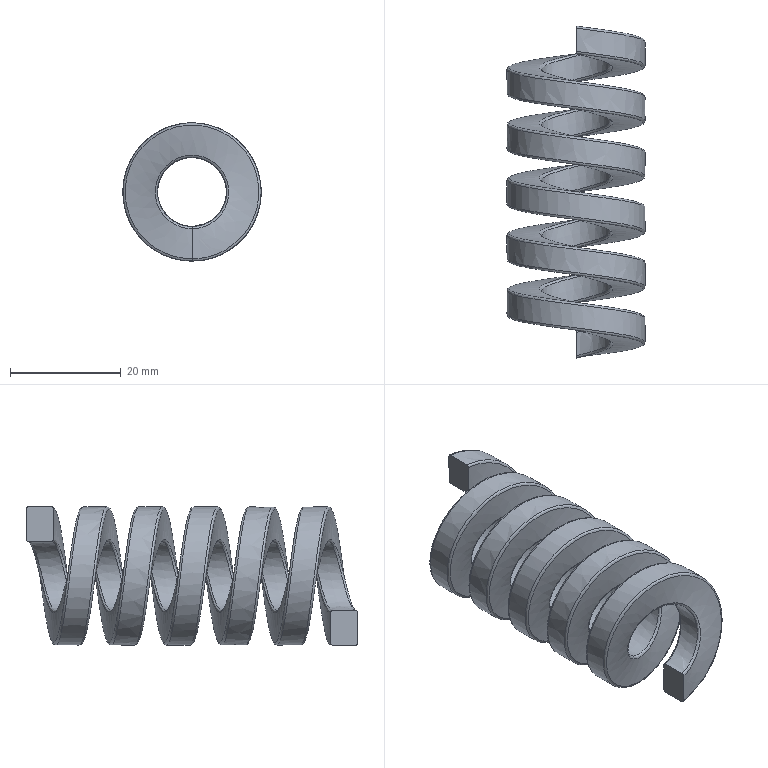Part | STEP file | solid 34 | 1 solid | 10 faces | box 25.029 x 60 x 25.037 mm | volume 10130 mm3 | spline 8 | plane 2